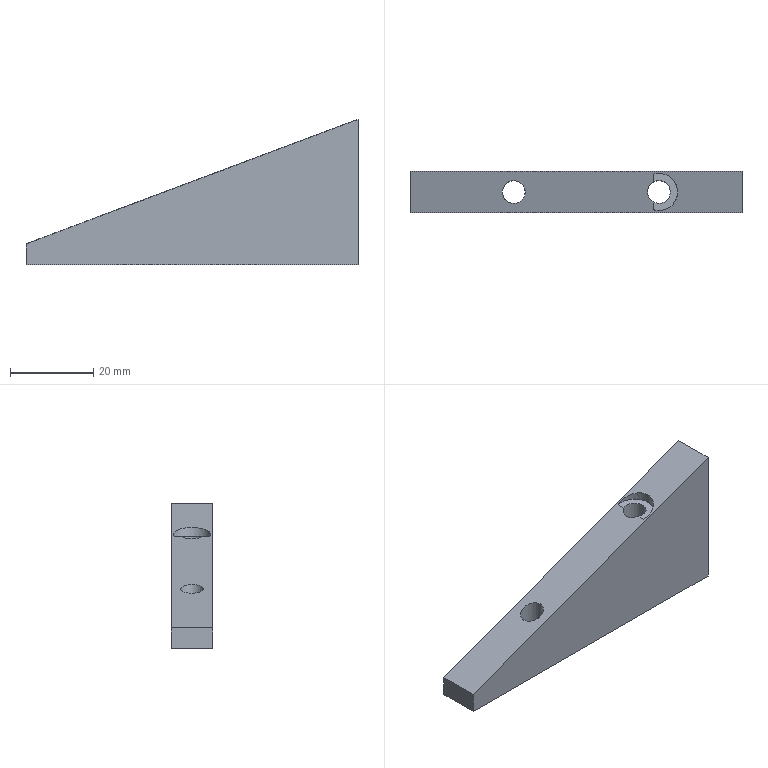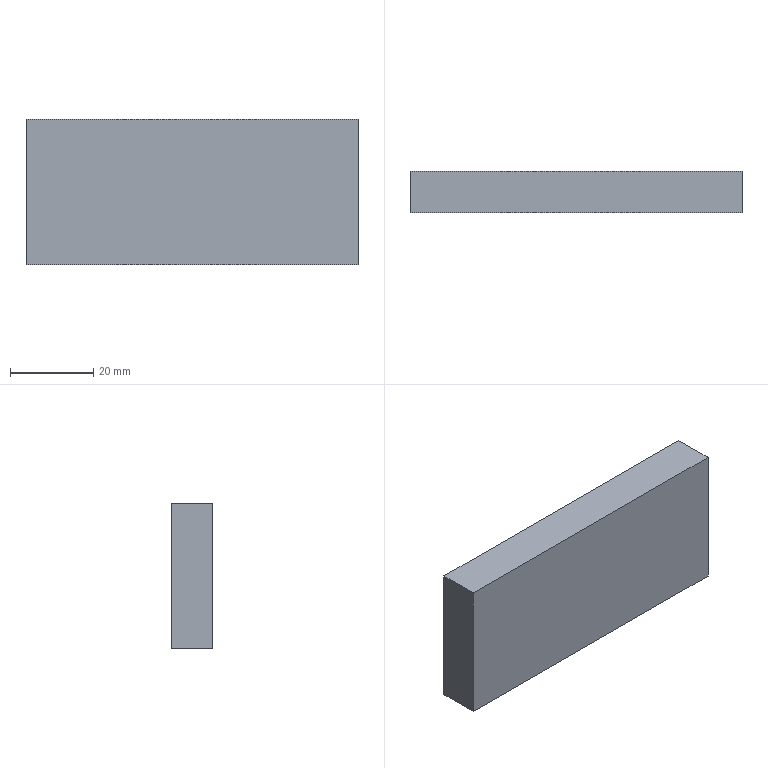CAM job | NX | 3+2 milling, drilling | part box 80 x 10 x 35 mm | stock box 80 x 10 x 35 mm
Tools:
number,name,description,diameter,corner_radius,flute_length,length,flutes
1,D10,Milling Tool-5 Parameters,10.0,0.0,50.0,75.0,2
0,D20,Milling Tool-5 Parameters,20.0,0.0,50.0,75.0,2
0,D6,Milling Tool-5 Parameters,6.0,0.0,50.0,75.0,2
0,D4,Milling Tool-5 Parameters,4.0,0.0,50.0,75.0,2
0,DR5.5,Drilling Tool,5.5,0.0,35.0,50.0,2
Operations:
program,operation,operation_type,tool,method,geometry_group,spindle_rpm,surface_speed,feed_per_tooth,feed_cut,feed_plunge,cut_length_mm,path_length_mm,cut_time_min,machine_time_min
NC_PROGRAM,FACE_MILLING,FaceMilling,D20,METHOD,WORKPIECE,0.0,0.0,0.0,250.0,100.0,707.0,896.111,2.828,2.847
NC_PROGRAM,PLANAR_PROFILE,PlanarMilling,D10,METHOD,WORKPIECE,0.0,0.0,0.0,250.0,100.0,5200.817,5384.003,20.803,20.822
NC_PROGRAM,PLANAR_MILL,PlanarMilling,D6,METHOD,WORKPIECE_1,0.0,0.0,0.0,250.0,100.0,140.533,607.693,0.5621,0.6088
NC_PROGRAM,PLANAR_MILL_1,PlanarMilling,D4,METHOD,WORKPIECE_1,0.0,0.0,0.0,250.0,100.0,36.602,125.397,0.1464,0.1553
NC_PROGRAM,PECK_DRILLING,Operation,DR5.5,METHOD,WORKPIECE_1,0.0,0.0,0.0,250.0,0.0,46.0,200.514,0.184,0.1995